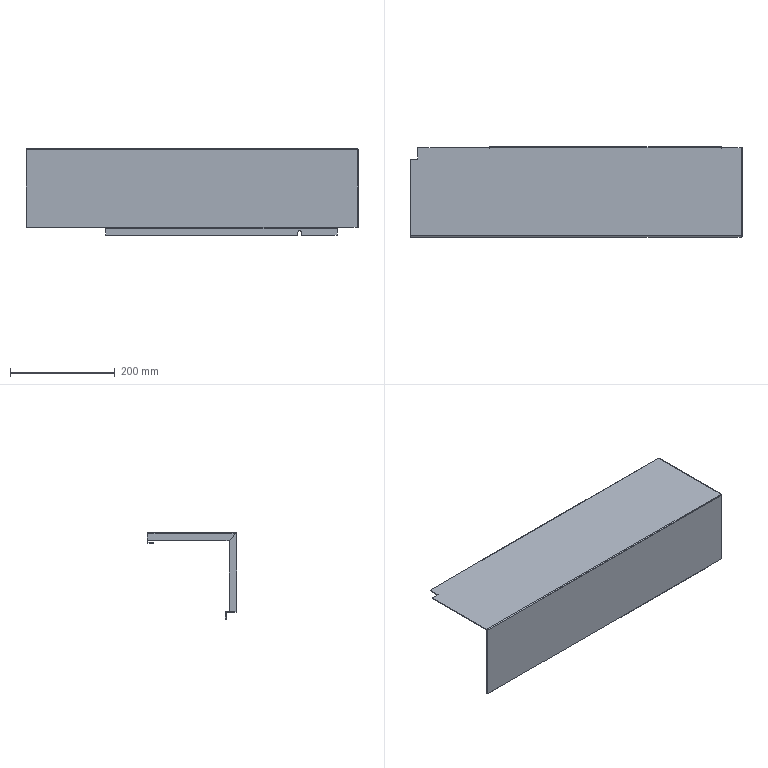Part | STEP file | FHD-021-001-C rack welded part C | 1 solid | 64 faces | box 633.5 x 171.5 x 165 mm | volume 350229 mm3 | plane 47 | cylinder 15 | spline 2 | commonest cylinder face diameters 0.4 x7 3.4 x7 6 x1